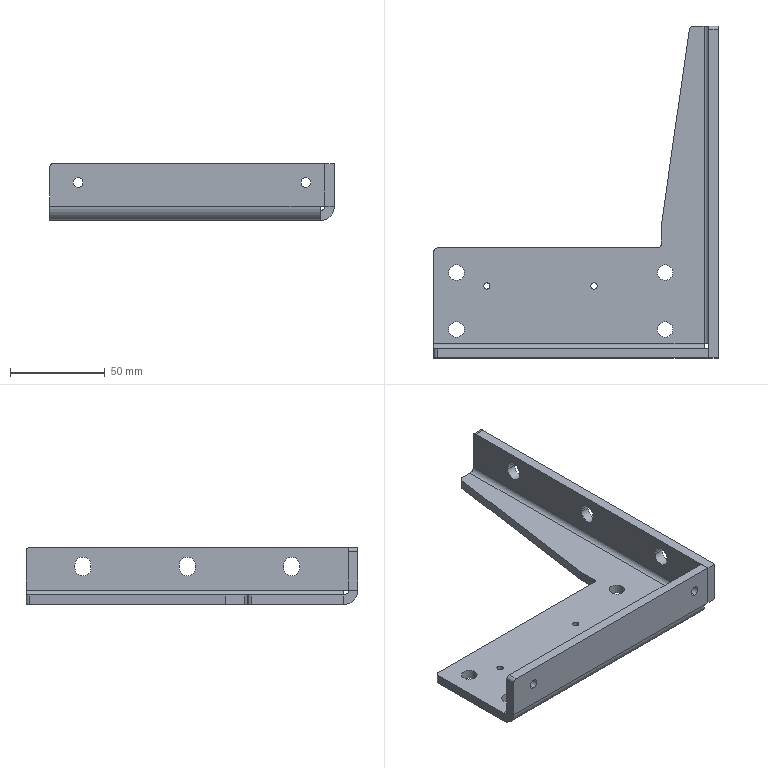Part | STEP file | 1 solid | 63 faces | box 150 x 175 x 30 mm | volume 90977 mm3 | cylinder 34 | plane 29 | commonest cylinder face diameters 8.5 x9 8.2 x8 5 x6 4 x5 3.3 x4 15 x2